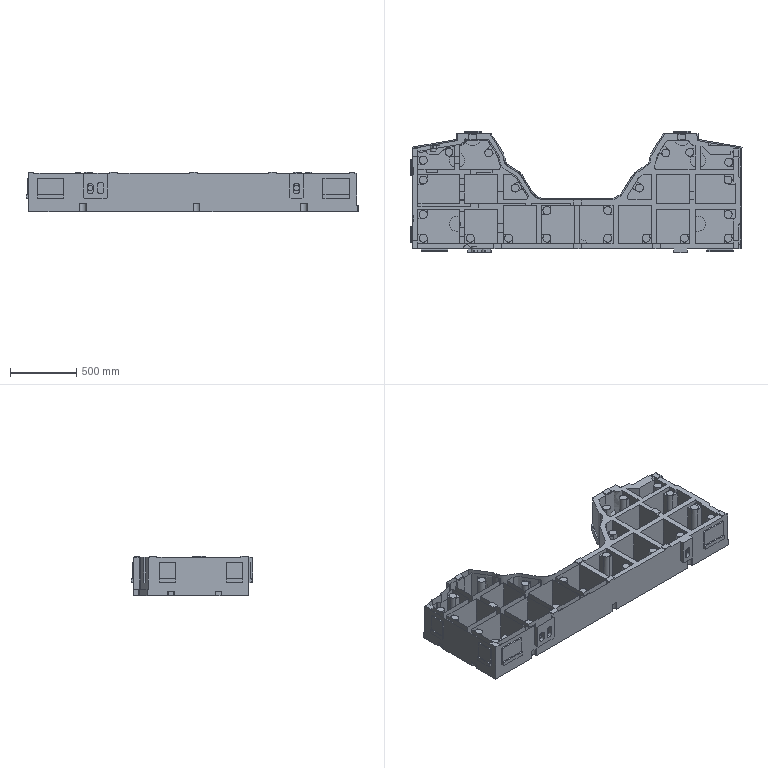Part | NX | features solid 2 | 1 solid | 667 faces | box 2510 x 920 x 300 mm | volume 226592805 mm3 | plane 535 | cylinder 93 | spline 39 | commonest cylinder face diameters 42 x24 60 x22 115 x12 40 x10 10 x6 50 x5